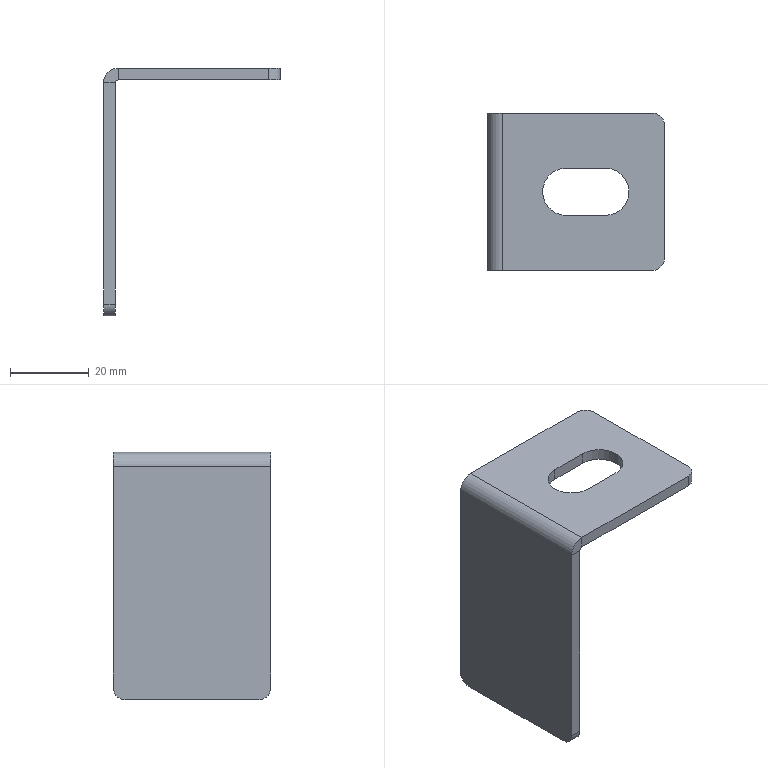Part | STEP file | 粉仓护栏FixedPlate 2 | 1 solid | 23 faces | box 45 x 40 x 63 mm | volume 11762 mm3 | plane 14 | cylinder 9 | commonest cylinder face diameters 6 x4 12 x3 1.473 x1 7.473 x1